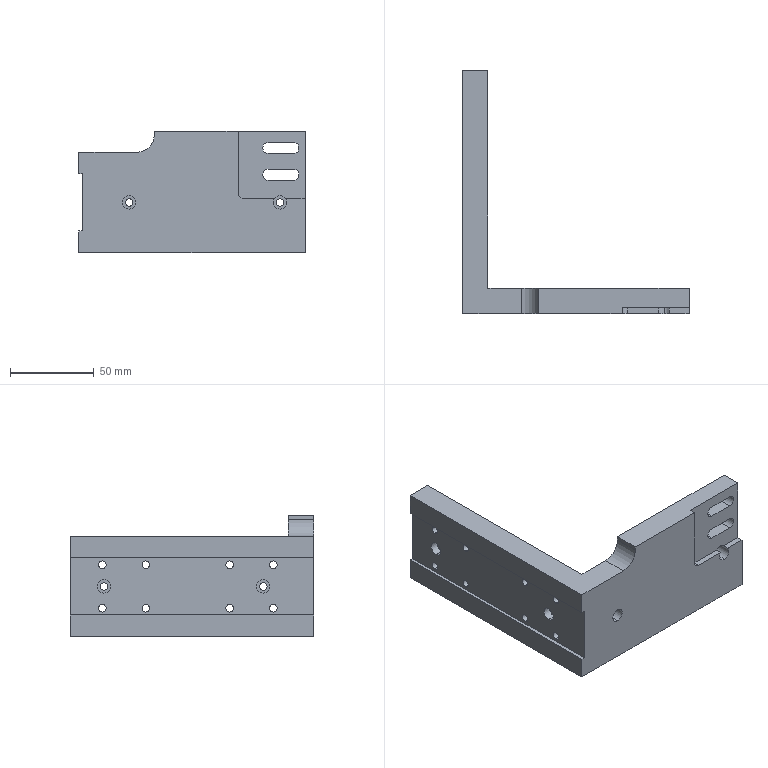Part | SolidWorks | features HoleWzd 4, ICE 4, Fillet 2, ExtruThin 1, Gusset 1 | 1 solid | 88 faces | box 135 x 145 x 72.5 mm | volume 232445 mm3 | cylinder 54 | plane 34 | commonest cylinder face diameters 4.5 x24 8 x24 6.6 x4 6 x1 20 x1